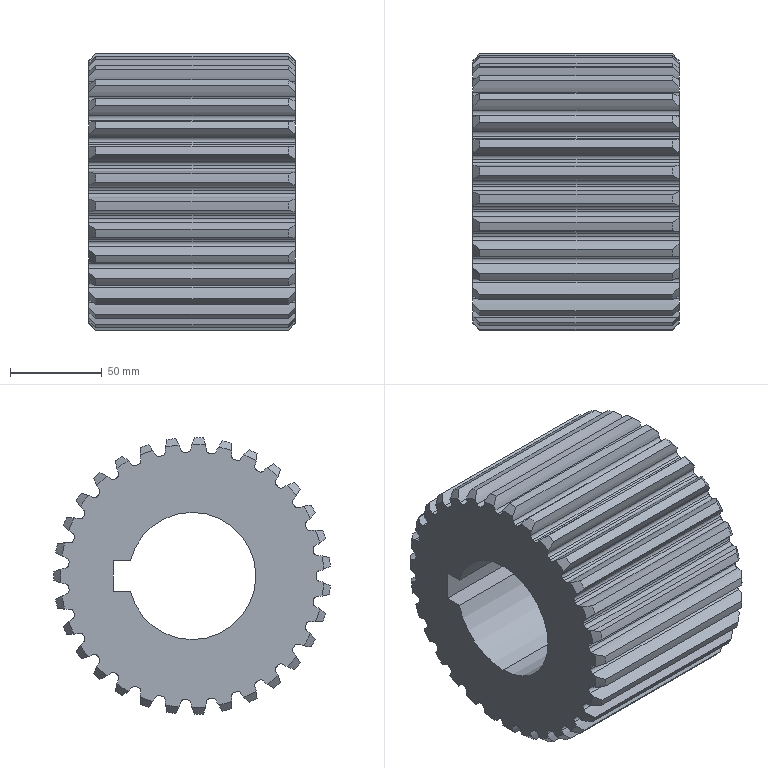Part | SolidWorks | features ICE 3, RevCut 1, Revolution 1, Scale 1 | 1 solid | 274 faces | box 112.5 x 150.753 x 150.909 mm | volume 1373452 mm3 | cylinder 205 | cone 64 | plane 5 | commonest cylinder face diameters 4.133 x75 48.325 x65 135 x31 150.938 x31 69.375 x3